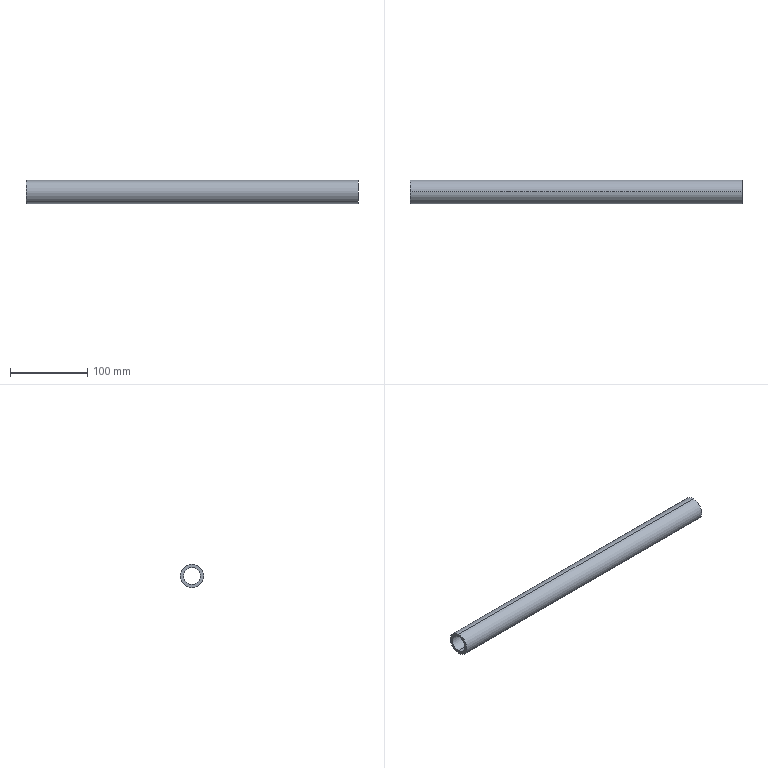Part | SolidWorks | features BaseBody 1, MoveFace 1 | 1 solid | 6 faces | box 429 x 30 x 30 mm | volume 140165 mm3 | cylinder 4 | plane 2 | commonest cylinder face diameters 22 x2 30 x2
STEP:
#1=CARTESIAN_POINT('',(429.,0.,15.));
#2=VERTEX_POINT('',#1);
#3=CARTESIAN_POINT('',(429.,0.,-15.));
#4=VERTEX_POINT('',#3);
#5=CARTESIAN_POINT('',(429.,0.,0.));
#6=DIRECTION('',(-1.,0.,0.));
#7=DIRECTION('',(0.,0.,1.));
#8=AXIS2_PLACEMENT_3D('',#5,#6,#7);
#9=CIRCLE('',#8,15.);
#10=EDGE_CURVE('',#2,#4,#9,.T.);
#11=ORIENTED_EDGE('',*,*,#10,.T.);
#12=CARTESIAN_POINT('',(0.,0.,-15.));
#13=VERTEX_POINT('',#12);
#14=CARTESIAN_POINT('',(0.,0.,-15.));
#15=DIRECTION('',(-1.,0.,0.));
#16=VECTOR('',#15,1000.);
#17=LINE('',#14,#16);
#18=EDGE_CURVE('',#4,#13,#17,.T.);
#19=ORIENTED_EDGE('',*,*,#18,.T.);
#20=CARTESIAN_POINT('',(0.,0.,15.));
#21=VERTEX_POINT('',#20);
#22=CARTESIAN_POINT('',(0.,0.,0.));
#23=DIRECTION('',(1.,0.,0.));
#24=DIRECTION('',(0.,0.,1.));
#25=AXIS2_PLACEMENT_3D('',#22,#23,#24);
#26=CIRCLE('',#25,15.);
#27=EDGE_CURVE('',#13,#21,#26,.T.);
#28=ORIENTED_EDGE('',*,*,#27,.T.);
#29=CARTESIAN_POINT('',(0.,0.,15.));
#30=DIRECTION('',(-1.,0.,0.));
#31=VECTOR('',#30,1000.);
#32=LINE('',#29,#31);
#33=EDGE_CURVE('',#2,#21,#32,.T.);
#34=ORIENTED_EDGE('',*,*,#33,.F.);
#35=EDGE_LOOP('',(#11,#19,#28,#34));
#36=FACE_OUTER_BOUND('',#35,.T.);
#37=CARTESIAN_POINT('',(0.,0.,0.));
#38=DIRECTION('',(-1.,0.,0.));
#39=DIRECTION('',(0.,0.,1.));
#40=AXIS2_PLACEMENT_3D('',#37,#38,#39);
#41=CYLINDRICAL_SURFACE('',#40,15.);
#42=ADVANCED_FACE('',(#36),#41,.T.);
#43=CARTESIAN_POINT('',(429.,0.,11.));
#44=VERTEX_POINT('',#43);
#45=CARTESIAN_POINT('',(429.,0.,-11.));
#46=VERTEX_POINT('',#45);
#47=CARTESIAN_POINT('',(429.,0.,0.));
#48=DIRECTION('',(1.,0.,0.));
#49=DIRECTION('',(0.,0.,1.));
#50=AXIS2_PLACEMENT_3D('',#47,#48,#49);
#51=CIRCLE('',#50,11.);
#52=EDGE_CURVE('',#44,#46,#51,.T.);
#53=ORIENTED_EDGE('',*,*,#52,.T.);
#54=CARTESIAN_POINT('',(0.,0.,-11.));
#55=VERTEX_POINT('',#54);
#56=CARTESIAN_POINT('',(0.,0.,-11.));
#57=DIRECTION('',(-1.,0.,0.));
#58=VECTOR('',#57,1000.);
#59=LINE('',#56,#58);
#60=EDGE_CURVE('',#46,#55,#59,.T.);
#61=ORIENTED_EDGE('',*,*,#60,.T.);
#62=CARTESIAN_POINT('',(0.,0.,11.));
#63=VERTEX_POINT('',#62);
#64=CARTESIAN_POINT('',(0.,0.,0.));
#65=DIRECTION('',(-1.,0.,0.));
#66=DIRECTION('',(0.,0.,1.));
#67=AXIS2_PLACEMENT_3D('',#64,#65,#66);
#68=CIRCLE('',#67,11.);
#69=EDGE_CURVE('',#55,#63,#68,.T.);
#70=ORIENTED_EDGE('',*,*,#69,.T.);
#71=CARTESIAN_POINT('',(0.,0.,11.));
#72=DIRECTION('',(-1.,0.,0.));
#73=VECTOR('',#72,1000.);
#74=LINE('',#71,#73);
#75=EDGE_CURVE('',#44,#63,#74,.T.);
#76=ORIENTED_EDGE('',*,*,#75,.F.);
#77=EDGE_LOOP('',(#53,#61,#70,#76));
#78=FACE_OUTER_BOUND('',#77,.T.);
#79=CARTESIAN_POINT('',(0.,0.,0.));
#80=DIRECTION('',(-1.,0.,0.));
#81=DIRECTION('',(0.,0.,1.));
#82=AXIS2_PLACEMENT_3D('',#79,#80,#81);
#83=CYLINDRICAL_SURFACE('',#82,11.);
#84=ADVANCED_FACE('',(#78),#83,.F.);
#85=ORIENTED_EDGE('',*,*,#18,.F.);
#86=CARTESIAN_POINT('',(429.,0.,0.));
#87=DIRECTION('',(-1.,0.,0.));
#88=DIRECTION('',(0.,0.,1.));
#89=AXIS2_PLACEMENT_3D('',#86,#87,#88);
#90=CIRCLE('',#89,15.);
#91=EDGE_CURVE('',#4,#2,#90,.T.);
#92=ORIENTED_EDGE('',*,*,#91,.T.);
#93=ORIENTED_EDGE('',*,*,#33,.T.);
#94=CARTESIAN_POINT('',(0.,0.,0.));
#95=DIRECTION('',(1.,0.,0.));
#96=DIRECTION('',(0.,0.,1.));
#97=AXIS2_PLACEMENT_3D('',#94,#95,#96);
#98=CIRCLE('',#97,15.);
#99=EDGE_CURVE('',#21,#13,#98,.T.);
#100=ORIENTED_EDGE('',*,*,#99,.T.);
#101=EDGE_LOOP('',(#85,#92,#93,#100));
#102=FACE_OUTER_BOUND('',#101,.T.);
#103=CARTESIAN_POINT('',(0.,0.,0.));
#104=DIRECTION('',(-1.,0.,0.));
#105=DIRECTION('',(0.,0.,1.));
#106=AXIS2_PLACEMENT_3D('',#103,#104,#105);
#107=CYLINDRICAL_SURFACE('',#106,15.);
#108=ADVANCED_FACE('',(#102),#107,.T.);
#109=ORIENTED_EDGE('',*,*,#99,.F.);
#110=ORIENTED_EDGE('',*,*,#27,.F.);
#111=EDGE_LOOP('',(#109,#110));
#112=FACE_OUTER_BOUND('',#111,.T.);
#113=CARTESIAN_POINT('',(0.,0.,0.));
#114=DIRECTION('',(-1.,0.,0.));
#115=DIRECTION('',(0.,0.,1.));
#116=AXIS2_PLACEMENT_3D('',#113,#114,#115);
#117=CIRCLE('',#116,11.);
#118=EDGE_CURVE('',#63,#55,#117,.T.);
#119=ORIENTED_EDGE('',*,*,#118,.F.);
#120=ORIENTED_EDGE('',*,*,#69,.F.);
#121=EDGE_LOOP('',(#119,#120));
#122=FACE_BOUND('',#121,.T.);
#123=CARTESIAN_POINT('',(0.,11.,0.));
#124=DIRECTION('',(1.,0.,0.));
#125=DIRECTION('',(0.,0.,-1.));
#126=AXIS2_PLACEMENT_3D('',#123,#124,#125);
#127=PLANE('',#126);
#128=ADVANCED_FACE('',(#112,#122),#127,.F.);
#129=ORIENTED_EDGE('',*,*,#52,.F.);
#130=CARTESIAN_POINT('',(429.,0.,0.));
#131=DIRECTION('',(1.,0.,0.));
#132=DIRECTION('',(0.,0.,1.));
#133=AXIS2_PLACEMENT_3D('',#130,#131,#132);
#134=CIRCLE('',#133,11.);
#135=EDGE_CURVE('',#46,#44,#134,.T.);
#136=ORIENTED_EDGE('',*,*,#135,.F.);
#137=EDGE_LOOP('',(#129,#136));
#138=FACE_BOUND('',#137,.T.);
#139=ORIENTED_EDGE('',*,*,#10,.F.);
#140=ORIENTED_EDGE('',*,*,#91,.F.);
#141=EDGE_LOOP('',(#139,#140));
#142=FACE_OUTER_BOUND('',#141,.T.);
#143=CARTESIAN_POINT('',(429.,15.,0.));
#144=DIRECTION('',(-1.,0.,0.));
#145=DIRECTION('',(0.,0.,1.));
#146=AXIS2_PLACEMENT_3D('',#143,#144,#145);
#147=PLANE('',#146);
#148=ADVANCED_FACE('',(#138,#142),#147,.F.);
#149=ORIENTED_EDGE('',*,*,#60,.F.);
#150=ORIENTED_EDGE('',*,*,#135,.T.);
#151=ORIENTED_EDGE('',*,*,#75,.T.);
#152=ORIENTED_EDGE('',*,*,#118,.T.);
#153=EDGE_LOOP('',(#149,#150,#151,#152));
#154=FACE_OUTER_BOUND('',#153,.T.);
#155=CARTESIAN_POINT('',(0.,0.,0.));
#156=DIRECTION('',(-1.,0.,0.));
#157=DIRECTION('',(0.,0.,1.));
#158=AXIS2_PLACEMENT_3D('',#155,#156,#157);
#159=CYLINDRICAL_SURFACE('',#158,11.);
#160=ADVANCED_FACE('',(#154),#159,.F.);
#161=CLOSED_SHELL('',(#42,#84,#108,#128,#148,#160));
#162=MANIFOLD_SOLID_BREP('',#161);
#163=CARTESIAN_POINT('',(0.,0.,0.));
#164=DIRECTION('',(0.,0.,1.));
#165=DIRECTION('',(1.,0.,0.));
#166=AXIS2_PLACEMENT_3D('',#163,#164,#165);
#167=(LENGTH_UNIT()NAMED_UNIT(*)SI_UNIT(.MILLI.,.METRE.));
#168=UNCERTAINTY_MEASURE_WITH_UNIT(LENGTH_MEASURE(0.00001),#167,'','');
#169=(NAMED_UNIT(*)PLANE_ANGLE_UNIT()SI_UNIT($,.RADIAN.));
#170=(NAMED_UNIT(*)SI_UNIT($,.STERADIAN.)SOLID_ANGLE_UNIT());
#171=(GEOMETRIC_REPRESENTATION_CONTEXT(3)GLOBAL_UNCERTAINTY_ASSIGNED_CONTEXT((#168))GLOBAL_UNIT_ASSIGNED_CONTEXT((#167,#169,#170))REPRESENTATION_CONTEXT('',''));
#172=ADVANCED_BREP_SHAPE_REPRESENTATION('',(#162,#166),#171);